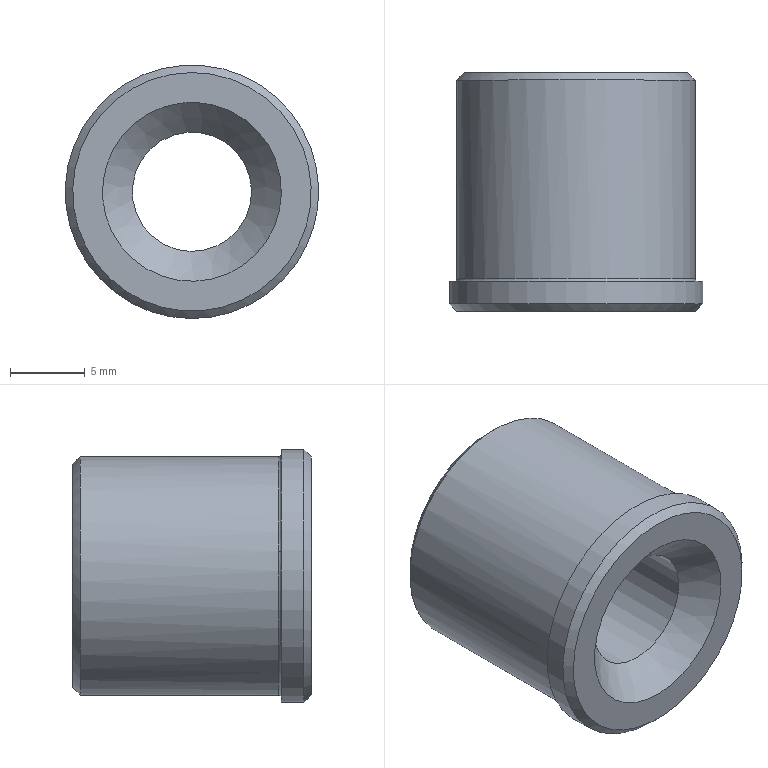Part | STEP file | PRODUTO_BUCHA | 1 solid | 13 faces | box 17 x 16 x 17 mm | volume 2259 mm3 | cylinder 4 | plane 4 | cone 3 | other 2 | commonest cylinder face diameters 8 x1 11 x1 16 x1 17 x1